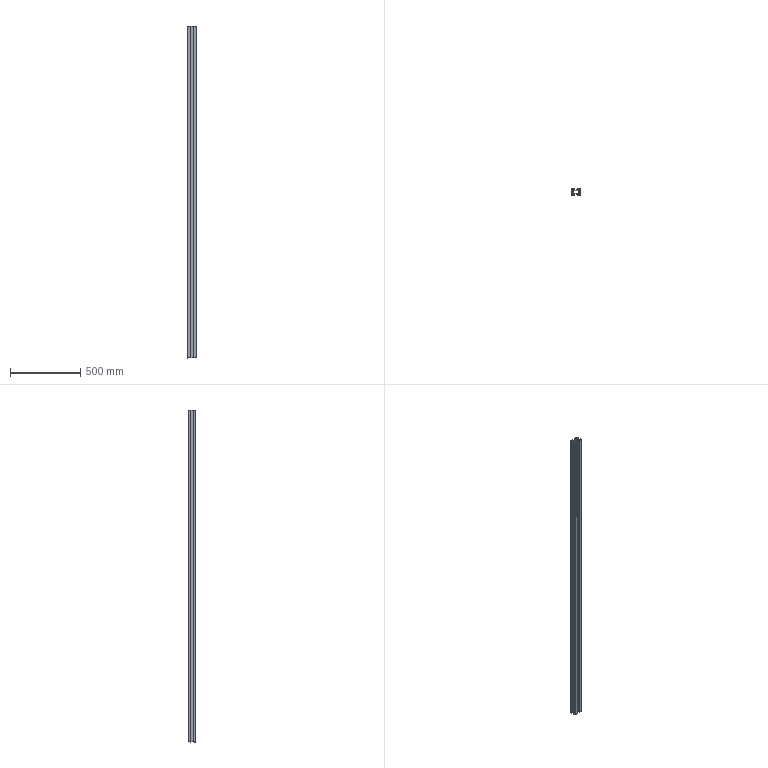Part | STEP file | 46A-00010CC11-2366mm | 1 solid | 143 faces | box 70 x 50 x 2366 mm | volume 1673926 mm3 | cylinder 85 | plane 58 | commonest cylinder face diameters 1 x25 4 x24 1.5 x16 3.7 x8 6.7 x8 2 x4